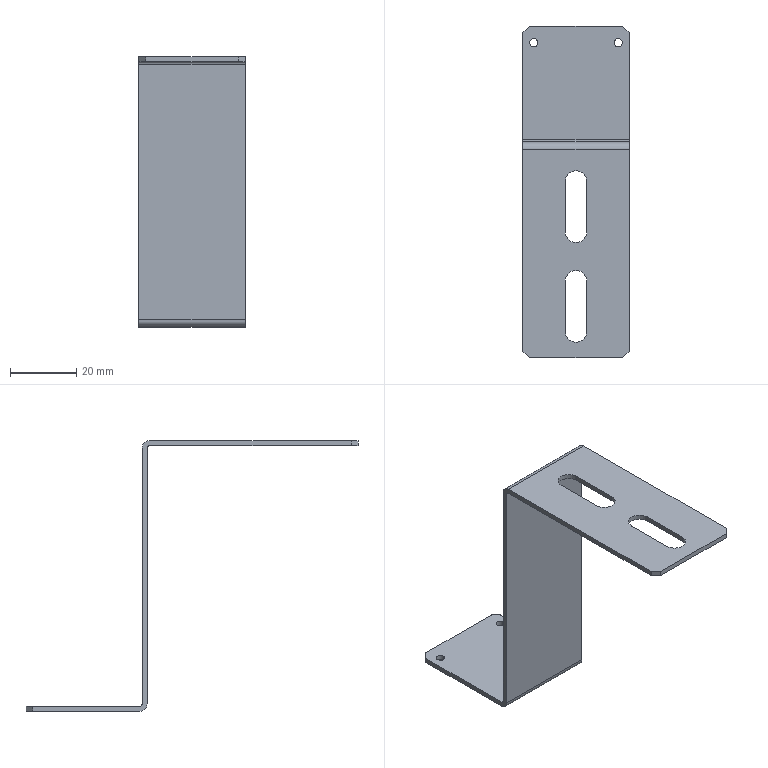Part | SolidWorks | features BaseBody 1 | 1 solid | 30 faces | box 32 x 100 x 81.5 mm | volume 8152 mm3 | plane 18 | cylinder 12 | commonest cylinder face diameters 2.5 x4 6.6 x4 1.473 x2 4.473 x2
STEP:
#1=CARTESIAN_POINT('',(11.45,95.,-80.));
#2=VERTEX_POINT('',#1);
#3=CARTESIAN_POINT('',(13.95,95.,-80.));
#4=VERTEX_POINT('',#3);
#5=CARTESIAN_POINT('',(12.7,95.,-80.));
#6=DIRECTION('',(0.,0.,1.));
#7=DIRECTION('',(1.,0.,0.));
#8=AXIS2_PLACEMENT_3D('',#5,#6,#7);
#9=CIRCLE('',#8,1.25);
#10=EDGE_CURVE('',#2,#4,#9,.T.);
#11=ORIENTED_EDGE('',*,*,#10,.T.);
#12=CARTESIAN_POINT('',(13.95,95.,-81.5));
#13=VERTEX_POINT('',#12);
#14=CARTESIAN_POINT('',(13.95,95.,-81.5));
#15=DIRECTION('',(0.,0.,-1.));
#16=VECTOR('',#15,1000.);
#17=LINE('',#14,#16);
#18=EDGE_CURVE('',#4,#13,#17,.T.);
#19=ORIENTED_EDGE('',*,*,#18,.T.);
#20=CARTESIAN_POINT('',(11.45,95.,-81.5));
#21=VERTEX_POINT('',#20);
#22=CARTESIAN_POINT('',(12.7,95.,-81.5));
#23=DIRECTION('',(0.,0.,-1.));
#24=DIRECTION('',(-1.,0.,0.));
#25=AXIS2_PLACEMENT_3D('',#22,#23,#24);
#26=CIRCLE('',#25,1.25);
#27=EDGE_CURVE('',#13,#21,#26,.T.);
#28=ORIENTED_EDGE('',*,*,#27,.T.);
#29=CARTESIAN_POINT('',(11.45,95.,-81.5));
#30=DIRECTION('',(0.,0.,-1.));
#31=VECTOR('',#30,1000.);
#32=LINE('',#29,#31);
#33=EDGE_CURVE('',#2,#21,#32,.T.);
#34=ORIENTED_EDGE('',*,*,#33,.F.);
#35=EDGE_LOOP('',(#11,#19,#28,#34));
#36=FACE_OUTER_BOUND('',#35,.T.);
#37=CARTESIAN_POINT('',(12.7,95.,-81.5));
#38=DIRECTION('',(0.,0.,-1.));
#39=DIRECTION('',(-1.,0.,0.));
#40=AXIS2_PLACEMENT_3D('',#37,#38,#39);
#41=CYLINDRICAL_SURFACE('',#40,1.25);
#42=ADVANCED_FACE('',(#36),#41,.F.);
#43=CARTESIAN_POINT('',(-13.95,95.,-80.));
#44=VERTEX_POINT('',#43);
#45=CARTESIAN_POINT('',(-11.45,95.,-80.));
#46=VERTEX_POINT('',#45);
#47=CARTESIAN_POINT('',(-12.7,95.,-80.));
#48=DIRECTION('',(0.,0.,1.));
#49=DIRECTION('',(1.,0.,0.));
#50=AXIS2_PLACEMENT_3D('',#47,#48,#49);
#51=CIRCLE('',#50,1.25);
#52=EDGE_CURVE('',#44,#46,#51,.T.);
#53=ORIENTED_EDGE('',*,*,#52,.T.);
#54=CARTESIAN_POINT('',(-11.45,95.,-81.5));
#55=VERTEX_POINT('',#54);
#56=CARTESIAN_POINT('',(-11.45,95.,-81.5));
#57=DIRECTION('',(0.,0.,-1.));
#58=VECTOR('',#57,1000.);
#59=LINE('',#56,#58);
#60=EDGE_CURVE('',#46,#55,#59,.T.);
#61=ORIENTED_EDGE('',*,*,#60,.T.);
#62=CARTESIAN_POINT('',(-13.95,95.,-81.5));
#63=VERTEX_POINT('',#62);
#64=CARTESIAN_POINT('',(-12.7,95.,-81.5));
#65=DIRECTION('',(0.,0.,-1.));
#66=DIRECTION('',(-1.,0.,0.));
#67=AXIS2_PLACEMENT_3D('',#64,#65,#66);
#68=CIRCLE('',#67,1.25);
#69=EDGE_CURVE('',#55,#63,#68,.T.);
#70=ORIENTED_EDGE('',*,*,#69,.T.);
#71=CARTESIAN_POINT('',(-13.95,95.,-81.5));
#72=DIRECTION('',(0.,0.,-1.));
#73=VECTOR('',#72,1000.);
#74=LINE('',#71,#73);
#75=EDGE_CURVE('',#44,#63,#74,.T.);
#76=ORIENTED_EDGE('',*,*,#75,.F.);
#77=EDGE_LOOP('',(#53,#61,#70,#76));
#78=FACE_OUTER_BOUND('',#77,.T.);
#79=CARTESIAN_POINT('',(-12.7,95.,-81.5));
#80=DIRECTION('',(0.,0.,-1.));
#81=DIRECTION('',(-1.,0.,0.));
#82=AXIS2_PLACEMENT_3D('',#79,#80,#81);
#83=CYLINDRICAL_SURFACE('',#82,1.25);
#84=ADVANCED_FACE('',(#78),#83,.F.);
#85=CARTESIAN_POINT('',(16.,98.,-80.));
#86=VERTEX_POINT('',#85);
#87=CARTESIAN_POINT('',(14.,100.,-80.));
#88=VERTEX_POINT('',#87);
#89=CARTESIAN_POINT('',(32.5,81.5,-80.));
#90=DIRECTION('',(-0.7071,0.7071,0.));
#91=VECTOR('',#90,1000.);
#92=LINE('',#89,#91);
#93=EDGE_CURVE('',#86,#88,#92,.T.);
#94=ORIENTED_EDGE('',*,*,#93,.F.);
#95=CARTESIAN_POINT('',(16.,98.,-81.5));
#96=VERTEX_POINT('',#95);
#97=CARTESIAN_POINT('',(16.,98.,-79.263));
#98=DIRECTION('',(0.,0.,1.));
#99=VECTOR('',#98,1000.);
#100=LINE('',#97,#99);
#101=EDGE_CURVE('',#96,#86,#100,.T.);
#102=ORIENTED_EDGE('',*,*,#101,.F.);
#103=CARTESIAN_POINT('',(14.,100.,-81.5));
#104=VERTEX_POINT('',#103);
#105=CARTESIAN_POINT('',(14.,100.,-81.5));
#106=DIRECTION('',(0.7071,-0.7071,0.));
#107=VECTOR('',#106,1000.);
#108=LINE('',#105,#107);
#109=EDGE_CURVE('',#104,#96,#108,.T.);
#110=ORIENTED_EDGE('',*,*,#109,.F.);
#111=CARTESIAN_POINT('',(14.,100.,-80.));
#112=DIRECTION('',(0.,0.,-1.));
#113=VECTOR('',#112,1000.);
#114=LINE('',#111,#113);
#115=EDGE_CURVE('',#88,#104,#114,.T.);
#116=ORIENTED_EDGE('',*,*,#115,.F.);
#117=EDGE_LOOP('',(#94,#102,#110,#116));
#118=FACE_OUTER_BOUND('',#117,.T.);
#119=CARTESIAN_POINT('',(14.,100.,-80.));
#120=DIRECTION('',(-0.7071,-0.7071,0.));
#121=DIRECTION('',(-0.7071,0.7071,0.));
#122=AXIS2_PLACEMENT_3D('',#119,#120,#121);
#123=PLANE('',#122);
#124=ADVANCED_FACE('',(#118),#123,.F.);
#125=CARTESIAN_POINT('',(-14.,100.,-80.));
#126=VERTEX_POINT('',#125);
#127=CARTESIAN_POINT('',(-16.,98.,-80.));
#128=VERTEX_POINT('',#127);
#129=CARTESIAN_POINT('',(-16.5,97.5,-80.));
#130=DIRECTION('',(-0.7071,-0.7071,0.));
#131=VECTOR('',#130,1000.);
#132=LINE('',#129,#131);
#133=EDGE_CURVE('',#126,#128,#132,.T.);
#134=ORIENTED_EDGE('',*,*,#133,.F.);
#135=CARTESIAN_POINT('',(-14.,100.,-81.5));
#136=VERTEX_POINT('',#135);
#137=CARTESIAN_POINT('',(-14.,100.,-80.));
#138=DIRECTION('',(0.,0.,1.));
#139=VECTOR('',#138,1000.);
#140=LINE('',#137,#139);
#141=EDGE_CURVE('',#136,#126,#140,.T.);
#142=ORIENTED_EDGE('',*,*,#141,.F.);
#143=CARTESIAN_POINT('',(-16.,98.,-81.5));
#144=VERTEX_POINT('',#143);
#145=CARTESIAN_POINT('',(-16.,98.,-81.5));
#146=DIRECTION('',(0.7071,0.7071,0.));
#147=VECTOR('',#146,1000.);
#148=LINE('',#145,#147);
#149=EDGE_CURVE('',#144,#136,#148,.T.);
#150=ORIENTED_EDGE('',*,*,#149,.F.);
#151=CARTESIAN_POINT('',(-16.,98.,-79.263));
#152=DIRECTION('',(0.,0.,-1.));
#153=VECTOR('',#152,1000.);
#154=LINE('',#151,#153);
#155=EDGE_CURVE('',#128,#144,#154,.T.);
#156=ORIENTED_EDGE('',*,*,#155,.F.);
#157=EDGE_LOOP('',(#134,#142,#150,#156));
#158=FACE_OUTER_BOUND('',#157,.T.);
#159=CARTESIAN_POINT('',(-16.,98.,-79.263));
#160=DIRECTION('',(0.7071,-0.7071,0.));
#161=DIRECTION('',(0.,0.,-1.));
#162=AXIS2_PLACEMENT_3D('',#159,#160,#161);
#163=PLANE('',#162);
#164=ADVANCED_FACE('',(#158),#163,.F.);
#165=CARTESIAN_POINT('',(-14.,0.,-1.5));
#166=VERTEX_POINT('',#165);
#167=CARTESIAN_POINT('',(-16.,2.,-1.5));
#168=VERTEX_POINT('',#167);
#169=CARTESIAN_POINT('',(-16.,2.,-1.5));
#170=DIRECTION('',(-0.7071,0.7071,0.));
#171=VECTOR('',#170,1000.);
#172=LINE('',#169,#171);
#173=EDGE_CURVE('',#166,#168,#172,.T.);
#174=ORIENTED_EDGE('',*,*,#173,.F.);
#175=CARTESIAN_POINT('',(-14.,0.,0.));
#176=VERTEX_POINT('',#175);
#177=CARTESIAN_POINT('',(-14.,0.,-1.5));
#178=DIRECTION('',(0.,0.,-1.));
#179=VECTOR('',#178,1000.);
#180=LINE('',#177,#179);
#181=EDGE_CURVE('',#176,#166,#180,.T.);
#182=ORIENTED_EDGE('',*,*,#181,.F.);
#183=CARTESIAN_POINT('',(-16.,2.,0.));
#184=VERTEX_POINT('',#183);
#185=CARTESIAN_POINT('',(1.,-15.,0.));
#186=DIRECTION('',(0.7071,-0.7071,0.));
#187=VECTOR('',#186,1000.);
#188=LINE('',#185,#187);
#189=EDGE_CURVE('',#184,#176,#188,.T.);
#190=ORIENTED_EDGE('',*,*,#189,.F.);
#191=CARTESIAN_POINT('',(-16.,2.,-2.237));
#192=DIRECTION('',(0.,0.,1.));
#193=VECTOR('',#192,1000.);
#194=LINE('',#191,#193);
#195=EDGE_CURVE('',#168,#184,#194,.T.);
#196=ORIENTED_EDGE('',*,*,#195,.F.);
#197=EDGE_LOOP('',(#174,#182,#190,#196));
#198=FACE_OUTER_BOUND('',#197,.T.);
#199=CARTESIAN_POINT('',(-16.,2.,-2.237));
#200=DIRECTION('',(0.7071,0.7071,0.));
#201=DIRECTION('',(0.,0.,-1.));
#202=AXIS2_PLACEMENT_3D('',#199,#200,#201);
#203=PLANE('',#202);
#204=ADVANCED_FACE('',(#198),#203,.F.);
#205=CARTESIAN_POINT('',(16.,2.,-1.5));
#206=VERTEX_POINT('',#205);
#207=CARTESIAN_POINT('',(14.,0.,-1.5));
#208=VERTEX_POINT('',#207);
#209=CARTESIAN_POINT('',(14.,0.,-1.5));
#210=DIRECTION('',(-0.7071,-0.7071,0.));
#211=VECTOR('',#210,1000.);
#212=LINE('',#209,#211);
#213=EDGE_CURVE('',#206,#208,#212,.T.);
#214=ORIENTED_EDGE('',*,*,#213,.F.);
#215=CARTESIAN_POINT('',(16.,2.,0.));
#216=VERTEX_POINT('',#215);
#217=CARTESIAN_POINT('',(16.,2.,-1.5));
#218=DIRECTION('',(0.,0.,-1.));
#219=VECTOR('',#218,1000.);
#220=LINE('',#217,#219);
#221=EDGE_CURVE('',#216,#206,#220,.T.);
#222=ORIENTED_EDGE('',*,*,#221,.F.);
#223=CARTESIAN_POINT('',(14.,0.,0.));
#224=VERTEX_POINT('',#223);
#225=CARTESIAN_POINT('',(15.,1.,0.));
#226=DIRECTION('',(0.7071,0.7071,0.));
#227=VECTOR('',#226,1000.);
#228=LINE('',#225,#227);
#229=EDGE_CURVE('',#224,#216,#228,.T.);
#230=ORIENTED_EDGE('',*,*,#229,.F.);
#231=CARTESIAN_POINT('',(14.,0.,0.));
#232=DIRECTION('',(0.,0.,1.));
#233=VECTOR('',#232,1000.);
#234=LINE('',#231,#233);
#235=EDGE_CURVE('',#208,#224,#234,.T.);
#236=ORIENTED_EDGE('',*,*,#235,.F.);
#237=EDGE_LOOP('',(#214,#222,#230,#236));
#238=FACE_OUTER_BOUND('',#237,.T.);
#239=CARTESIAN_POINT('',(14.,0.,-1.5));
#240=DIRECTION('',(0.7071,-0.7071,0.));
#241=DIRECTION('',(0.,0.,-1.));
#242=AXIS2_PLACEMENT_3D('',#239,#240,#241);
#243=PLANE('',#242);
#244=ADVANCED_FACE('',(#238),#243,.T.);
#245=CARTESIAN_POINT('',(-3.3,38.,0.));
#246=VERTEX_POINT('',#245);
#247=CARTESIAN_POINT('',(-3.3,38.,-1.5));
#248=VERTEX_POINT('',#247);
#249=CARTESIAN_POINT('',(-3.3,38.,0.001));
#250=DIRECTION('',(0.,0.,-1.));
#251=VECTOR('',#250,1000.);
#252=LINE('',#249,#251);
#253=EDGE_CURVE('',#246,#248,#252,.T.);
#254=ORIENTED_EDGE('',*,*,#253,.T.);
#255=CARTESIAN_POINT('',(-3.3,53.,-1.5));
#256=VERTEX_POINT('',#255);
#257=CARTESIAN_POINT('',(-3.3,38.,-1.5));
#258=DIRECTION('',(0.,1.,0.));
#259=VECTOR('',#258,1000.);
#260=LINE('',#257,#259);
#261=EDGE_CURVE('',#248,#256,#260,.T.);
#262=ORIENTED_EDGE('',*,*,#261,.T.);
#263=CARTESIAN_POINT('',(-3.3,53.,0.));
#264=VERTEX_POINT('',#263);
#265=CARTESIAN_POINT('',(-3.3,53.,0.001));
#266=DIRECTION('',(0.,0.,-1.));
#267=VECTOR('',#266,1000.);
#268=LINE('',#265,#267);
#269=EDGE_CURVE('',#264,#256,#268,.T.);
#270=ORIENTED_EDGE('',*,*,#269,.F.);
#271=CARTESIAN_POINT('',(-3.3,38.,0.));
#272=DIRECTION('',(0.,1.,0.));
#273=VECTOR('',#272,1000.);
#274=LINE('',#271,#273);
#275=EDGE_CURVE('',#246,#264,#274,.T.);
#276=ORIENTED_EDGE('',*,*,#275,.F.);
#277=EDGE_LOOP('',(#254,#262,#270,#276));
#278=FACE_OUTER_BOUND('',#277,.T.);
#279=CARTESIAN_POINT('',(-3.3,38.,0.001));
#280=DIRECTION('',(-1.,0.,0.));
#281=DIRECTION('',(0.,0.,1.));
#282=AXIS2_PLACEMENT_3D('',#279,#280,#281);
#283=PLANE('',#282);
#284=ADVANCED_FACE('',(#278),#283,.F.);
#285=ORIENTED_EDGE('',*,*,#269,.T.);
#286=CARTESIAN_POINT('',(3.3,53.,-1.5));
#287=VERTEX_POINT('',#286);
#288=CARTESIAN_POINT('',(0.,53.,-1.5));
#289=DIRECTION('',(0.,0.,-1.));
#290=DIRECTION('',(-1.,0.,0.));
#291=AXIS2_PLACEMENT_3D('',#288,#289,#290);
#292=CIRCLE('',#291,3.3);
#293=EDGE_CURVE('',#256,#287,#292,.T.);
#294=ORIENTED_EDGE('',*,*,#293,.T.);
#295=CARTESIAN_POINT('',(3.3,53.,0.));
#296=VERTEX_POINT('',#295);
#297=CARTESIAN_POINT('',(3.3,53.,0.001));
#298=DIRECTION('',(0.,0.,-1.));
#299=VECTOR('',#298,1000.);
#300=LINE('',#297,#299);
#301=EDGE_CURVE('',#296,#287,#300,.T.);
#302=ORIENTED_EDGE('',*,*,#301,.F.);
#303=CARTESIAN_POINT('',(0.,53.,0.));
#304=DIRECTION('',(0.,0.,-1.));
#305=DIRECTION('',(1.,0.,0.));
#306=AXIS2_PLACEMENT_3D('',#303,#304,#305);
#307=CIRCLE('',#306,3.3);
#308=EDGE_CURVE('',#264,#296,#307,.T.);
#309=ORIENTED_EDGE('',*,*,#308,.F.);
#310=EDGE_LOOP('',(#285,#294,#302,#309));
#311=FACE_OUTER_BOUND('',#310,.T.);
#312=CARTESIAN_POINT('',(0.,53.,0.001));
#313=DIRECTION('',(0.,0.,-1.));
#314=DIRECTION('',(-1.,0.,0.));
#315=AXIS2_PLACEMENT_3D('',#312,#313,#314);
#316=CYLINDRICAL_SURFACE('',#315,3.3);
#317=ADVANCED_FACE('',(#311),#316,.F.);
#318=ORIENTED_EDGE('',*,*,#301,.T.);
#319=CARTESIAN_POINT('',(3.3,38.,-1.5));
#320=VERTEX_POINT('',#319);
#321=CARTESIAN_POINT('',(3.3,38.,-1.5));
#322=DIRECTION('',(0.,-1.,0.));
#323=VECTOR('',#322,1000.);
#324=LINE('',#321,#323);
#325=EDGE_CURVE('',#287,#320,#324,.T.);
#326=ORIENTED_EDGE('',*,*,#325,.T.);
#327=CARTESIAN_POINT('',(3.3,38.,0.));
#328=VERTEX_POINT('',#327);
#329=CARTESIAN_POINT('',(3.3,38.,0.001));
#330=DIRECTION('',(0.,0.,-1.));
#331=VECTOR('',#330,1000.);
#332=LINE('',#329,#331);
#333=EDGE_CURVE('',#328,#320,#332,.T.);
#334=ORIENTED_EDGE('',*,*,#333,.F.);
#335=CARTESIAN_POINT('',(3.3,38.,0.));
#336=DIRECTION('',(0.,-1.,0.));
#337=VECTOR('',#336,1000.);
#338=LINE('',#335,#337);
#339=EDGE_CURVE('',#296,#328,#338,.T.);
#340=ORIENTED_EDGE('',*,*,#339,.F.);
#341=EDGE_LOOP('',(#318,#326,#334,#340));
#342=FACE_OUTER_BOUND('',#341,.T.);
#343=CARTESIAN_POINT('',(3.3,38.,0.001));
#344=DIRECTION('',(1.,0.,0.));
#345=DIRECTION('',(0.,1.,0.));
#346=AXIS2_PLACEMENT_3D('',#343,#344,#345);
#347=PLANE('',#346);
#348=ADVANCED_FACE('',(#342),#347,.F.);
#349=ORIENTED_EDGE('',*,*,#333,.T.);
#350=CARTESIAN_POINT('',(0.,38.,-1.5));
#351=DIRECTION('',(0.,0.,-1.));
#352=DIRECTION('',(-1.,0.,0.));
#353=AXIS2_PLACEMENT_3D('',#350,#351,#352);
#354=CIRCLE('',#353,3.3);
#355=EDGE_CURVE('',#320,#248,#354,.T.);
#356=ORIENTED_EDGE('',*,*,#355,.T.);
#357=ORIENTED_EDGE('',*,*,#253,.F.);
#358=CARTESIAN_POINT('',(0.,38.,0.));
#359=DIRECTION('',(0.,0.,-1.));
#360=DIRECTION('',(1.,0.,0.));
#361=AXIS2_PLACEMENT_3D('',#358,#359,#360);
#362=CIRCLE('',#361,3.3);
#363=EDGE_CURVE('',#328,#246,#362,.T.);
#364=ORIENTED_EDGE('',*,*,#363,.F.);
#365=EDGE_LOOP('',(#349,#356,#357,#364));
#366=FACE_OUTER_BOUND('',#365,.T.);
#367=CARTESIAN_POINT('',(0.,38.,0.001));
#368=DIRECTION('',(0.,0.,-1.));
#369=DIRECTION('',(-1.,0.,0.));
#370=AXIS2_PLACEMENT_3D('',#367,#368,#369);
#371=CYLINDRICAL_SURFACE('',#370,3.3);
#372=ADVANCED_FACE('',(#366),#371,.F.);
#373=CARTESIAN_POINT('',(-3.3,8.,0.));
#374=VERTEX_POINT('',#373);
#375=CARTESIAN_POINT('',(-3.3,8.,-1.5));
#376=VERTEX_POINT('',#375);
#377=CARTESIAN_POINT('',(-3.3,8.,0.001));
#378=DIRECTION('',(0.,0.,-1.));
#379=VECTOR('',#378,1000.);
#380=LINE('',#377,#379);
#381=EDGE_CURVE('',#374,#376,#380,.T.);
#382=ORIENTED_EDGE('',*,*,#381,.T.);
#383=CARTESIAN_POINT('',(-3.3,23.,-1.5));
#384=VERTEX_POINT('',#383);
#385=CARTESIAN_POINT('',(-3.3,8.,-1.5));
#386=DIRECTION('',(0.,1.,0.));
#387=VECTOR('',#386,1000.);
#388=LINE('',#385,#387);
#389=EDGE_CURVE('',#376,#384,#388,.T.);
#390=ORIENTED_EDGE('',*,*,#389,.T.);
#391=CARTESIAN_POINT('',(-3.3,23.,0.));
#392=VERTEX_POINT('',#391);
#393=CARTESIAN_POINT('',(-3.3,23.,0.001));
#394=DIRECTION('',(0.,0.,-1.));
#395=VECTOR('',#394,1000.);
#396=LINE('',#393,#395);
#397=EDGE_CURVE('',#392,#384,#396,.T.);
#398=ORIENTED_EDGE('',*,*,#397,.F.);
#399=CARTESIAN_POINT('',(-3.3,8.,0.));
#400=DIRECTION('',(0.,1.,0.));
#401=VECTOR('',#400,1000.);
#402=LINE('',#399,#401);
#403=EDGE_CURVE('',#374,#392,#402,.T.);
#404=ORIENTED_EDGE('',*,*,#403,.F.);
#405=EDGE_LOOP('',(#382,#390,#398,#404));
#406=FACE_OUTER_BOUND('',#405,.T.);
#407=CARTESIAN_POINT('',(-3.3,8.,0.001));
#408=DIRECTION('',(-1.,0.,0.));
#409=DIRECTION('',(0.,0.,1.));
#410=AXIS2_PLACEMENT_3D('',#407,#408,#409);
#411=PLANE('',#410);
#412=ADVANCED_FACE('',(#406),#411,.F.);
#413=ORIENTED_EDGE('',*,*,#397,.T.);
#414=CARTESIAN_POINT('',(3.3,23.,-1.5));
#415=VERTEX_POINT('',#414);
#416=CARTESIAN_POINT('',(0.,23.,-1.5));
#417=DIRECTION('',(0.,0.,-1.));
#418=DIRECTION('',(-1.,0.,0.));
#419=AXIS2_PLACEMENT_3D('',#416,#417,#418);
#420=CIRCLE('',#419,3.3);
#421=EDGE_CURVE('',#384,#415,#420,.T.);
#422=ORIENTED_EDGE('',*,*,#421,.T.);
#423=CARTESIAN_POINT('',(3.3,23.,0.));
#424=VERTEX_POINT('',#423);
#425=CARTESIAN_POINT('',(3.3,23.,0.001));
#426=DIRECTION('',(0.,0.,-1.));
#427=VECTOR('',#426,1000.);
#428=LINE('',#425,#427);
#429=EDGE_CURVE('',#424,#415,#428,.T.);
#430=ORIENTED_EDGE('',*,*,#429,.F.);
#431=CARTESIAN_POINT('',(0.,23.,0.));
#432=DIRECTION('',(0.,0.,-1.));
#433=DIRECTION('',(1.,0.,0.));
#434=AXIS2_PLACEMENT_3D('',#431,#432,#433);
#435=CIRCLE('',#434,3.3);
#436=EDGE_CURVE('',#392,#424,#435,.T.);
#437=ORIENTED_EDGE('',*,*,#436,.F.);
#438=EDGE_LOOP('',(#413,#422,#430,#437));
#439=FACE_OUTER_BOUND('',#438,.T.);
#440=CARTESIAN_POINT('',(0.,23.,0.001));
#441=DIRECTION('',(0.,0.,-1.));
#442=DIRECTION('',(-1.,0.,0.));
#443=AXIS2_PLACEMENT_3D('',#440,#441,#442);
#444=CYLINDRICAL_SURFACE('',#443,3.3);
#445=ADVANCED_FACE('',(#439),#444,.F.);
#446=ORIENTED_EDGE('',*,*,#429,.T.);
#447=CARTESIAN_POINT('',(3.3,8.,-1.5));
#448=VERTEX_POINT('',#447);
#449=CARTESIAN_POINT('',(3.3,8.,-1.5));
#450=DIRECTION('',(0.,-1.,0.));
#451=VECTOR('',#450,1000.);
#452=LINE('',#449,#451);
#453=EDGE_CURVE('',#415,#448,#452,.T.);
#454=ORIENTED_EDGE('',*,*,#453,.T.);
#455=CARTESIAN_POINT('',(3.3,8.,0.));
#456=VERTEX_POINT('',#455);
#457=CARTESIAN_POINT('',(3.3,8.,0.001));
#458=DIRECTION('',(0.,0.,-1.));
#459=VECTOR('',#458,1000.);
#460=LINE('',#457,#459);
#461=EDGE_CURVE('',#456,#448,#460,.T.);
#462=ORIENTED_EDGE('',*,*,#461,.F.);
#463=CARTESIAN_POINT('',(3.3,8.,0.));
#464=DIRECTION('',(0.,-1.,0.));
#465=VECTOR('',#464,1000.);
#466=LINE('',#463,#465);
#467=EDGE_CURVE('',#424,#456,#466,.T.);
#468=ORIENTED_EDGE('',*,*,#467,.F.);
#469=EDGE_LOOP('',(#446,#454,#462,#468));
#470=FACE_OUTER_BOUND('',#469,.T.);
#471=CARTESIAN_POINT('',(3.3,8.,0.001));
#472=DIRECTION('',(1.,0.,0.));
#473=DIRECTION('',(0.,1.,0.));
#474=AXIS2_PLACEMENT_3D('',#471,#472,#473);
#475=PLANE('',#474);
#476=ADVANCED_FACE('',(#470),#475,.F.);
#477=ORIENTED_EDGE('',*,*,#461,.T.);
#478=CARTESIAN_POINT('',(0.,8.,-1.5));
#479=DIRECTION('',(0.,0.,-1.));
#480=DIRECTION('',(-1.,0.,0.));
#481=AXIS2_PLACEMENT_3D('',#478,#479,#480);
#482=CIRCLE('',#481,3.3);
#483=EDGE_CURVE('',#448,#376,#482,.T.);
#484=ORIENTED_EDGE('',*,*,#483,.T.);
#485=ORIENTED_EDGE('',*,*,#381,.F.);
#486=CARTESIAN_POINT('',(0.,8.,0.));
#487=DIRECTION('',(0.,0.,-1.));
#488=DIRECTION('',(1.,0.,0.));
#489=AXIS2_PLACEMENT_3D('',#486,#487,#488);
#490=CIRCLE('',#489,3.3);
#491=EDGE_CURVE('',#456,#374,#490,.T.);
#492=ORIENTED_EDGE('',*,*,#491,.F.);
#493=EDGE_LOOP('',(#477,#484,#485,#492));
#494=FACE_OUTER_BOUND('',#493,.T.);
#495=CARTESIAN_POINT('',(0.,8.,0.001));
#496=DIRECTION('',(0.,0.,-1.));
#497=DIRECTION('',(-1.,0.,0.));
#498=AXIS2_PLACEMENT_3D('',#495,#496,#497);
#499=CYLINDRICAL_SURFACE('',#498,3.3);
#500=ADVANCED_FACE('',(#494),#499,.F.);
#501=CARTESIAN_POINT('',(-16.,63.5,-79.263));
#502=VERTEX_POINT('',#501);
#503=CARTESIAN_POINT('',(-16.,65.737,-81.5));
#504=VERTEX_POINT('',#503);
#505=CARTESIAN_POINT('',(-16.,65.737,-79.263));
#506=DIRECTION('',(1.,0.,0.));
#507=DIRECTION('',(0.,0.,-1.));
#508=AXIS2_PLACEMENT_3D('',#505,#506,#507);
#509=CIRCLE('',#508,2.237);
#510=EDGE_CURVE('',#502,#504,#509,.T.);
#511=ORIENTED_EDGE('',*,*,#510,.T.);
#512=CARTESIAN_POINT('',(16.,65.737,-81.5));
#513=VERTEX_POINT('',#512);
#514=CARTESIAN_POINT('',(16.,65.737,-81.5));
#515=DIRECTION('',(-1.,0.,0.));
#516=VECTOR('',#515,1000.);
#517=LINE('',#514,#516);
#518=EDGE_CURVE('',#513,#504,#517,.T.);
#519=ORIENTED_EDGE('',*,*,#518,.F.);
#520=CARTESIAN_POINT('',(16.,63.5,-79.263));
#521=VERTEX_POINT('',#520);
#522=CARTESIAN_POINT('',(16.,65.737,-79.263));
#523=DIRECTION('',(1.,0.,0.));
#524=DIRECTION('',(0.,0.,-1.));
#525=AXIS2_PLACEMENT_3D('',#522,#523,#524);
#526=CIRCLE('',#525,2.237);
#527=EDGE_CURVE('',#521,#513,#526,.T.);
#528=ORIENTED_EDGE('',*,*,#527,.F.);
#529=CARTESIAN_POINT('',(16.,63.5,-79.263));
#530=DIRECTION('',(-1.,0.,0.));
#531=VECTOR('',#530,1000.);
#532=LINE('',#529,#531);
#533=EDGE_CURVE('',#521,#502,#532,.T.);
#534=ORIENTED_EDGE('',*,*,#533,.T.);
#535=EDGE_LOOP('',(#511,#519,#528,#534));
#536=FACE_OUTER_BOUND('',#535,.T.);
#537=CARTESIAN_POINT('',(16.,65.737,-79.263));
#538=DIRECTION('',(-1.,0.,0.));
#539=DIRECTION('',(0.,0.,1.));
#540=AXIS2_PLACEMENT_3D('',#537,#538,#539);
#541=CYLINDRICAL_SURFACE('',#540,2.237);
#542=ADVANCED_FACE('',(#536),#541,.T.);
#543=CARTESIAN_POINT('',(-16.,63.5,-2.237));
#544=VERTEX_POINT('',#543);
#545=CARTESIAN_POINT('',(-16.,63.5,0.));
#546=DIRECTION('',(0.,0.,-1.));
#547=VECTOR('',#546,1000.);
#548=LINE('',#545,#547);
#549=EDGE_CURVE('',#544,#502,#548,.T.);
#550=ORIENTED_EDGE('',*,*,#549,.T.);
#551=ORIENTED_EDGE('',*,*,#533,.F.);
#552=CARTESIAN_POINT('',(16.,63.5,-2.237));
#553=VERTEX_POINT('',#552);
#554=CARTESIAN_POINT('',(16.,63.5,0.));
#555=DIRECTION('',(0.,0.,-1.));
#556=VECTOR('',#555,1000.);
#557=LINE('',#554,#556);
#558=EDGE_CURVE('',#553,#521,#557,.T.);
#559=ORIENTED_EDGE('',*,*,#558,.F.);
#560=CARTESIAN_POINT('',(16.,63.5,-2.237));
#561=DIRECTION('',(-1.,0.,0.));
#562=VECTOR('',#561,1000.);
#563=LINE('',#560,#562);
#564=EDGE_CURVE('',#553,#544,#563,.T.);
#565=ORIENTED_EDGE('',*,*,#564,.T.);
#566=EDGE_LOOP('',(#550,#551,#559,#565));
#567=FACE_OUTER_BOUND('',#566,.T.);
#568=CARTESIAN_POINT('',(16.,63.5,0.));
#569=DIRECTION('',(0.,1.,0.));
#570=DIRECTION('',(1.,0.,0.));
#571=AXIS2_PLACEMENT_3D('',#568,#569,#570);
#572=PLANE('',#571);
#573=ADVANCED_FACE('',(#567),#572,.F.);
#574=CARTESIAN_POINT('',(-16.,62.763,-1.5));
#575=VERTEX_POINT('',#574);
#576=CARTESIAN_POINT('',(-16.,62.763,-2.237));
#577=DIRECTION('',(-1.,0.,0.));
#578=DIRECTION('',(0.,0.,-1.));
#579=AXIS2_PLACEMENT_3D('',#576,#577,#578);
#580=CIRCLE('',#579,0.7366);
#581=EDGE_CURVE('',#575,#544,#580,.T.);
#582=ORIENTED_EDGE('',*,*,#581,.T.);
#583=ORIENTED_EDGE('',*,*,#564,.F.);
#584=CARTESIAN_POINT('',(16.,62.763,-1.5));
#585=VERTEX_POINT('',#584);
#586=CARTESIAN_POINT('',(16.,62.763,-2.237));
#587=DIRECTION('',(-1.,0.,0.));
#588=DIRECTION('',(0.,0.,-1.));
#589=AXIS2_PLACEMENT_3D('',#586,#587,#588);
#590=CIRCLE('',#589,0.7366);
#591=EDGE_CURVE('',#585,#553,#590,.T.);
#592=ORIENTED_EDGE('',*,*,#591,.F.);
#593=CARTESIAN_POINT('',(16.,62.763,-1.5));
#594=DIRECTION('',(-1.,0.,0.));
#595=VECTOR('',#594,1000.);
#596=LINE('',#593,#595);
#597=EDGE_CURVE('',#585,#575,#596,.T.);
#598=ORIENTED_EDGE('',*,*,#597,.T.);
#599=EDGE_LOOP('',(#582,#583,#592,#598));
#600=FACE_OUTER_BOUND('',#599,.T.);
#601=CARTESIAN_POINT('',(16.,62.763,-2.237));
#602=DIRECTION('',(-1.,0.,0.));
#603=DIRECTION('',(0.,0.,1.));
#604=AXIS2_PLACEMENT_3D('',#601,#602,#603);
#605=CYLINDRICAL_SURFACE('',#604,0.7366);
#606=ADVANCED_FACE('',(#600),#605,.F.);
#607=ORIENTED_EDGE('',*,*,#389,.F.);
#608=ORIENTED_EDGE('',*,*,#483,.F.);
#609=ORIENTED_EDGE('',*,*,#453,.F.);
#610=ORIENTED_EDGE('',*,*,#421,.F.);
#611=EDGE_LOOP('',(#607,#608,#609,#610));
#612=FACE_BOUND('',#611,.T.);
#613=ORIENTED_EDGE('',*,*,#261,.F.);
#614=ORIENTED_EDGE('',*,*,#355,.F.);
#615=ORIENTED_EDGE('',*,*,#325,.F.);
#616=ORIENTED_EDGE('',*,*,#293,.F.);
#617=EDGE_LOOP('',(#613,#614,#615,#616));
#618=FACE_BOUND('',#617,.T.);
#619=CARTESIAN_POINT('',(16.,0.,-1.5));
#620=DIRECTION('',(0.,1.,0.));
#621=VECTOR('',#620,1000.);
#622=LINE('',#619,#621);
#623=EDGE_CURVE('',#206,#585,#622,.T.);
#624=ORIENTED_EDGE('',*,*,#623,.F.);
#625=ORIENTED_EDGE('',*,*,#213,.T.);
#626=CARTESIAN_POINT('',(16.,0.,-1.5));
#627=DIRECTION('',(-1.,0.,0.));
#628=VECTOR('',#627,1000.);
#629=LINE('',#626,#628);
#630=EDGE_CURVE('',#208,#166,#629,.T.);
#631=ORIENTED_EDGE('',*,*,#630,.T.);
#632=ORIENTED_EDGE('',*,*,#173,.T.);
#633=CARTESIAN_POINT('',(-16.,0.,-1.5));
#634=DIRECTION('',(0.,1.,0.));
#635=VECTOR('',#634,1000.);
#636=LINE('',#633,#635);
#637=EDGE_CURVE('',#168,#575,#636,.T.);
#638=ORIENTED_EDGE('',*,*,#637,.T.);
#639=ORIENTED_EDGE('',*,*,#597,.F.);
#640=EDGE_LOOP('',(#624,#625,#631,#632,#638,#639));
#641=FACE_OUTER_BOUND('',#640,.T.);
#642=CARTESIAN_POINT('',(16.,0.,-1.5));
#643=DIRECTION('',(0.,0.,1.));
#644=DIRECTION('',(1.,0.,0.));
#645=AXIS2_PLACEMENT_3D('',#642,#643,#644);
#646=PLANE('',#645);
#647=ADVANCED_FACE('',(#612,#618,#641),#646,.F.);
#648=ORIENTED_EDGE('',*,*,#630,.F.);
#649=ORIENTED_EDGE('',*,*,#235,.T.);
#650=CARTESIAN_POINT('',(16.,0.,0.));
#651=DIRECTION('',(-1.,0.,0.));
#652=VECTOR('',#651,1000.);
#653=LINE('',#650,#652);
#654=EDGE_CURVE('',#224,#176,#653,.T.);
#655=ORIENTED_EDGE('',*,*,#654,.T.);
#656=ORIENTED_EDGE('',*,*,#181,.T.);
#657=EDGE_LOOP('',(#648,#649,#655,#656));
#658=FACE_OUTER_BOUND('',#657,.T.);
#659=CARTESIAN_POINT('',(16.,0.,-1.5));
#660=DIRECTION('',(0.,-1.,0.));
#661=DIRECTION('',(0.,0.,-1.));
#662=AXIS2_PLACEMENT_3D('',#659,#660,#661);
#663=PLANE('',#662);
#664=ADVANCED_FACE('',(#658),#663,.T.);
#665=ORIENTED_EDGE('',*,*,#491,.T.);
#666=ORIENTED_EDGE('',*,*,#403,.T.);
#667=ORIENTED_EDGE('',*,*,#436,.T.);
#668=ORIENTED_EDGE('',*,*,#467,.T.);
#669=EDGE_LOOP('',(#665,#666,#667,#668));
#670=FACE_BOUND('',#669,.T.);
#671=ORIENTED_EDGE('',*,*,#363,.T.);
#672=ORIENTED_EDGE('',*,*,#275,.T.);
#673=ORIENTED_EDGE('',*,*,#308,.T.);
#674=ORIENTED_EDGE('',*,*,#339,.T.);
#675=EDGE_LOOP('',(#671,#672,#673,#674));
#676=FACE_BOUND('',#675,.T.);
#677=ORIENTED_EDGE('',*,*,#654,.F.);
#678=ORIENTED_EDGE('',*,*,#229,.T.);
#679=CARTESIAN_POINT('',(16.,62.763,0.));
#680=VERTEX_POINT('',#679);
#681=CARTESIAN_POINT('',(16.,0.,0.));
#682=DIRECTION('',(0.,1.,0.));
#683=VECTOR('',#682,1000.);
#684=LINE('',#681,#683);
#685=EDGE_CURVE('',#216,#680,#684,.T.);
#686=ORIENTED_EDGE('',*,*,#685,.T.);
#687=CARTESIAN_POINT('',(-16.,62.763,0.));
#688=VERTEX_POINT('',#687);
#689=CARTESIAN_POINT('',(16.,62.763,0.));
#690=DIRECTION('',(-1.,0.,0.));
#691=VECTOR('',#690,1000.);
#692=LINE('',#689,#691);
#693=EDGE_CURVE('',#680,#688,#692,.T.);
#694=ORIENTED_EDGE('',*,*,#693,.T.);
#695=CARTESIAN_POINT('',(-16.,0.,0.));
#696=DIRECTION('',(0.,1.,0.));
#697=VECTOR('',#696,1000.);
#698=LINE('',#695,#697);
#699=EDGE_CURVE('',#184,#688,#698,.T.);
#700=ORIENTED_EDGE('',*,*,#699,.F.);
#701=ORIENTED_EDGE('',*,*,#189,.T.);
#702=EDGE_LOOP('',(#677,#678,#686,#694,#700,#701));
#703=FACE_OUTER_BOUND('',#702,.T.);
#704=CARTESIAN_POINT('',(16.,0.,0.));
#705=DIRECTION('',(0.,0.,1.));
#706=DIRECTION('',(1.,0.,0.));
#707=AXIS2_PLACEMENT_3D('',#704,#705,#706);
#708=PLANE('',#707);
#709=ADVANCED_FACE('',(#670,#676,#703),#708,.T.);
#710=CARTESIAN_POINT('',(-16.,65.,-2.237));
#711=VERTEX_POINT('',#710);
#712=CARTESIAN_POINT('',(-16.,62.763,-2.237));
#713=DIRECTION('',(-1.,0.,0.));
#714=DIRECTION('',(0.,0.,-1.));
#715=AXIS2_PLACEMENT_3D('',#712,#713,#714);
#716=CIRCLE('',#715,2.237);
#717=EDGE_CURVE('',#688,#711,#716,.T.);
#718=ORIENTED_EDGE('',*,*,#717,.F.);
#719=ORIENTED_EDGE('',*,*,#693,.F.);
#720=CARTESIAN_POINT('',(16.,65.,-2.237));
#721=VERTEX_POINT('',#720);
#722=CARTESIAN_POINT('',(16.,62.763,-2.237));
#723=DIRECTION('',(-1.,0.,0.));
#724=DIRECTION('',(0.,0.,-1.));
#725=AXIS2_PLACEMENT_3D('',#722,#723,#724);
#726=CIRCLE('',#725,2.237);
#727=EDGE_CURVE('',#680,#721,#726,.T.);
#728=ORIENTED_EDGE('',*,*,#727,.T.);
#729=CARTESIAN_POINT('',(16.,65.,-2.237));
#730=DIRECTION('',(-1.,0.,0.));
#731=VECTOR('',#730,1000.);
#732=LINE('',#729,#731);
#733=EDGE_CURVE('',#721,#711,#732,.T.);
#734=ORIENTED_EDGE('',*,*,#733,.T.);
#735=EDGE_LOOP('',(#718,#719,#728,#734));
#736=FACE_OUTER_BOUND('',#735,.T.);
#737=CARTESIAN_POINT('',(16.,62.763,-2.237));
#738=DIRECTION('',(-1.,0.,0.));
#739=DIRECTION('',(0.,0.,1.));
#740=AXIS2_PLACEMENT_3D('',#737,#738,#739);
#741=CYLINDRICAL_SURFACE('',#740,2.237);
#742=ADVANCED_FACE('',(#736),#741,.T.);
#743=CARTESIAN_POINT('',(-16.,65.,-79.263));
#744=VERTEX_POINT('',#743);
#745=CARTESIAN_POINT('',(-16.,65.,0.));
#746=DIRECTION('',(0.,0.,-1.));
#747=VECTOR('',#746,1000.);
#748=LINE('',#745,#747);
#749=EDGE_CURVE('',#711,#744,#748,.T.);
#750=ORIENTED_EDGE('',*,*,#749,.F.);
#751=ORIENTED_EDGE('',*,*,#733,.F.);
#752=CARTESIAN_POINT('',(16.,65.,-79.263));
#753=VERTEX_POINT('',#752);
#754=CARTESIAN_POINT('',(16.,65.,0.));
#755=DIRECTION('',(0.,0.,-1.));
#756=VECTOR('',#755,1000.);
#757=LINE('',#754,#756);
#758=EDGE_CURVE('',#721,#753,#757,.T.);
#759=ORIENTED_EDGE('',*,*,#758,.T.);
#760=CARTESIAN_POINT('',(16.,65.,-79.263));
#761=DIRECTION('',(-1.,0.,0.));
#762=VECTOR('',#761,1000.);
#763=LINE('',#760,#762);
#764=EDGE_CURVE('',#753,#744,#763,.T.);
#765=ORIENTED_EDGE('',*,*,#764,.T.);
#766=EDGE_LOOP('',(#750,#751,#759,#765));
#767=FACE_OUTER_BOUND('',#766,.T.);
#768=CARTESIAN_POINT('',(16.,65.,0.));
#769=DIRECTION('',(0.,1.,0.));
#770=DIRECTION('',(1.,0.,0.));
#771=AXIS2_PLACEMENT_3D('',#768,#769,#770);
#772=PLANE('',#771);
#773=ADVANCED_FACE('',(#767),#772,.T.);
#774=CARTESIAN_POINT('',(-16.,65.737,-80.));
#775=VERTEX_POINT('',#774);
#776=CARTESIAN_POINT('',(-16.,65.737,-79.263));
#777=DIRECTION('',(1.,0.,0.));
#778=DIRECTION('',(0.,0.,1.));
#779=AXIS2_PLACEMENT_3D('',#776,#777,#778);
#780=CIRCLE('',#779,0.7366);
#781=EDGE_CURVE('',#744,#775,#780,.T.);
#782=ORIENTED_EDGE('',*,*,#781,.F.);
#783=ORIENTED_EDGE('',*,*,#764,.F.);
#784=CARTESIAN_POINT('',(16.,65.737,-80.));
#785=VERTEX_POINT('',#784);
#786=CARTESIAN_POINT('',(16.,65.737,-79.263));
#787=DIRECTION('',(1.,0.,0.));
#788=DIRECTION('',(0.,0.,1.));
#789=AXIS2_PLACEMENT_3D('',#786,#787,#788);
#790=CIRCLE('',#789,0.7366);
#791=EDGE_CURVE('',#753,#785,#790,.T.);
#792=ORIENTED_EDGE('',*,*,#791,.T.);
#793=CARTESIAN_POINT('',(16.,65.737,-80.));
#794=DIRECTION('',(-1.,0.,0.));
#795=VECTOR('',#794,1000.);
#796=LINE('',#793,#795);
#797=EDGE_CURVE('',#785,#775,#796,.T.);
#798=ORIENTED_EDGE('',*,*,#797,.T.);
#799=EDGE_LOOP('',(#782,#783,#792,#798));
#800=FACE_OUTER_BOUND('',#799,.T.);
#801=CARTESIAN_POINT('',(16.,65.737,-79.263));
#802=DIRECTION('',(-1.,0.,0.));
#803=DIRECTION('',(0.,0.,1.));
#804=AXIS2_PLACEMENT_3D('',#801,#802,#803);
#805=CYLINDRICAL_SURFACE('',#804,0.7366);
#806=ADVANCED_FACE('',(#800),#805,.F.);
#807=ORIENTED_EDGE('',*,*,#52,.F.);
#808=CARTESIAN_POINT('',(-12.7,95.,-80.));
#809=DIRECTION('',(0.,0.,1.));
#810=DIRECTION('',(1.,0.,0.));
#811=AXIS2_PLACEMENT_3D('',#808,#809,#810);
#812=CIRCLE('',#811,1.25);
#813=EDGE_CURVE('',#46,#44,#812,.T.);
#814=ORIENTED_EDGE('',*,*,#813,.F.);
#815=EDGE_LOOP('',(#807,#814));
#816=FACE_BOUND('',#815,.T.);
#817=ORIENTED_EDGE('',*,*,#10,.F.);
#818=CARTESIAN_POINT('',(12.7,95.,-80.));
#819=DIRECTION('',(0.,0.,1.));
#820=DIRECTION('',(1.,0.,0.));
#821=AXIS2_PLACEMENT_3D('',#818,#819,#820);
#822=CIRCLE('',#821,1.25);
#823=EDGE_CURVE('',#4,#2,#822,.T.);
#824=ORIENTED_EDGE('',*,*,#823,.F.);
#825=EDGE_LOOP('',(#817,#824));
#826=FACE_BOUND('',#825,.T.);
#827=CARTESIAN_POINT('',(16.,100.,-80.));
#828=DIRECTION('',(-1.,0.,0.));
#829=VECTOR('',#828,1000.);
#830=LINE('',#827,#829);
#831=EDGE_CURVE('',#88,#126,#830,.T.);
#832=ORIENTED_EDGE('',*,*,#831,.T.);
#833=ORIENTED_EDGE('',*,*,#133,.T.);
#834=CARTESIAN_POINT('',(-16.,65.,-80.));
#835=DIRECTION('',(0.,1.,0.));
#836=VECTOR('',#835,1000.);
#837=LINE('',#834,#836);
#838=EDGE_CURVE('',#775,#128,#837,.T.);
#839=ORIENTED_EDGE('',*,*,#838,.F.);
#840=ORIENTED_EDGE('',*,*,#797,.F.);
#841=CARTESIAN_POINT('',(16.,65.,-80.));
#842=DIRECTION('',(0.,1.,0.));
#843=VECTOR('',#842,1000.);
#844=LINE('',#841,#843);
#845=EDGE_CURVE('',#785,#86,#844,.T.);
#846=ORIENTED_EDGE('',*,*,#845,.T.);
#847=ORIENTED_EDGE('',*,*,#93,.T.);
#848=EDGE_LOOP('',(#832,#833,#839,#840,#846,#847));
#849=FACE_OUTER_BOUND('',#848,.T.);
#850=CARTESIAN_POINT('',(16.,65.,-80.));
#851=DIRECTION('',(0.,0.,1.));
#852=DIRECTION('',(1.,0.,0.));
#853=AXIS2_PLACEMENT_3D('',#850,#851,#852);
#854=PLANE('',#853);
#855=ADVANCED_FACE('',(#816,#826,#849),#854,.T.);
#856=CARTESIAN_POINT('',(16.,100.,-81.5));
#857=DIRECTION('',(-1.,0.,0.));
#858=VECTOR('',#857,1000.);
#859=LINE('',#856,#858);
#860=EDGE_CURVE('',#104,#136,#859,.T.);
#861=ORIENTED_EDGE('',*,*,#860,.T.);
#862=ORIENTED_EDGE('',*,*,#141,.T.);
#863=ORIENTED_EDGE('',*,*,#831,.F.);
#864=ORIENTED_EDGE('',*,*,#115,.T.);
#865=EDGE_LOOP('',(#861,#862,#863,#864));
#866=FACE_OUTER_BOUND('',#865,.T.);
#867=CARTESIAN_POINT('',(16.,100.,-80.));
#868=DIRECTION('',(0.,1.,0.));
#869=DIRECTION('',(1.,0.,0.));
#870=AXIS2_PLACEMENT_3D('',#867,#868,#869);
#871=PLANE('',#870);
#872=ADVANCED_FACE('',(#866),#871,.T.);
#873=CARTESIAN_POINT('',(-12.7,95.,-81.5));
#874=DIRECTION('',(0.,0.,-1.));
#875=DIRECTION('',(-1.,0.,0.));
#876=AXIS2_PLACEMENT_3D('',#873,#874,#875);
#877=CIRCLE('',#876,1.25);
#878=EDGE_CURVE('',#63,#55,#877,.T.);
#879=ORIENTED_EDGE('',*,*,#878,.F.);
#880=ORIENTED_EDGE('',*,*,#69,.F.);
#881=EDGE_LOOP('',(#879,#880));
#882=FACE_BOUND('',#881,.T.);
#883=CARTESIAN_POINT('',(12.7,95.,-81.5));
#884=DIRECTION('',(0.,0.,-1.));
#885=DIRECTION('',(-1.,0.,0.));
#886=AXIS2_PLACEMENT_3D('',#883,#884,#885);
#887=CIRCLE('',#886,1.25);
#888=EDGE_CURVE('',#21,#13,#887,.T.);
#889=ORIENTED_EDGE('',*,*,#888,.F.);
#890=ORIENTED_EDGE('',*,*,#27,.F.);
#891=EDGE_LOOP('',(#889,#890));
#892=FACE_BOUND('',#891,.T.);
#893=CARTESIAN_POINT('',(-16.,65.,-81.5));
#894=DIRECTION('',(0.,1.,0.));
#895=VECTOR('',#894,1000.);
#896=LINE('',#893,#895);
#897=EDGE_CURVE('',#504,#144,#896,.T.);
#898=ORIENTED_EDGE('',*,*,#897,.T.);
#899=ORIENTED_EDGE('',*,*,#149,.T.);
#900=ORIENTED_EDGE('',*,*,#860,.F.);
#901=ORIENTED_EDGE('',*,*,#109,.T.);
#902=CARTESIAN_POINT('',(16.,65.,-81.5));
#903=DIRECTION('',(0.,1.,0.));
#904=VECTOR('',#903,1000.);
#905=LINE('',#902,#904);
#906=EDGE_CURVE('',#513,#96,#905,.T.);
#907=ORIENTED_EDGE('',*,*,#906,.F.);
#908=ORIENTED_EDGE('',*,*,#518,.T.);
#909=EDGE_LOOP('',(#898,#899,#900,#901,#907,#908));
#910=FACE_OUTER_BOUND('',#909,.T.);
#911=CARTESIAN_POINT('',(16.,65.,-81.5));
#912=DIRECTION('',(0.,0.,1.));
#913=DIRECTION('',(1.,0.,0.));
#914=AXIS2_PLACEMENT_3D('',#911,#912,#913);
#915=PLANE('',#914);
#916=ADVANCED_FACE('',(#882,#892,#910),#915,.F.);
#917=ORIENTED_EDGE('',*,*,#581,.F.);
#918=ORIENTED_EDGE('',*,*,#637,.F.);
#919=ORIENTED_EDGE('',*,*,#195,.T.);
#920=ORIENTED_EDGE('',*,*,#699,.T.);
#921=ORIENTED_EDGE('',*,*,#717,.T.);
#922=ORIENTED_EDGE('',*,*,#749,.T.);
#923=ORIENTED_EDGE('',*,*,#781,.T.);
#924=ORIENTED_EDGE('',*,*,#838,.T.);
#925=ORIENTED_EDGE('',*,*,#155,.T.);
#926=ORIENTED_EDGE('',*,*,#897,.F.);
#927=ORIENTED_EDGE('',*,*,#510,.F.);
#928=ORIENTED_EDGE('',*,*,#549,.F.);
#929=EDGE_LOOP('',(#917,#918,#919,#920,#921,#922,#923,#924,#925,#926,#927,#928));
#930=FACE_OUTER_BOUND('',#929,.T.);
#931=CARTESIAN_POINT('',(-16.,62.763,0.));
#932=DIRECTION('',(-1.,0.,0.));
#933=DIRECTION('',(0.,0.,1.));
#934=AXIS2_PLACEMENT_3D('',#931,#932,#933);
#935=PLANE('',#934);
#936=ADVANCED_FACE('',(#930),#935,.T.);
#937=ORIENTED_EDGE('',*,*,#591,.T.);
#938=ORIENTED_EDGE('',*,*,#558,.T.);
#939=ORIENTED_EDGE('',*,*,#527,.T.);
#940=ORIENTED_EDGE('',*,*,#906,.T.);
#941=ORIENTED_EDGE('',*,*,#101,.T.);
#942=ORIENTED_EDGE('',*,*,#845,.F.);
#943=ORIENTED_EDGE('',*,*,#791,.F.);
#944=ORIENTED_EDGE('',*,*,#758,.F.);
#945=ORIENTED_EDGE('',*,*,#727,.F.);
#946=ORIENTED_EDGE('',*,*,#685,.F.);
#947=ORIENTED_EDGE('',*,*,#221,.T.);
#948=ORIENTED_EDGE('',*,*,#623,.T.);
#949=EDGE_LOOP('',(#937,#938,#939,#940,#941,#942,#943,#944,#945,#946,#947,#948));
#950=FACE_OUTER_BOUND('',#949,.T.);
#951=CARTESIAN_POINT('',(16.,65.,-2.237));
#952=DIRECTION('',(1.,0.,0.));
#953=DIRECTION('',(0.,1.,0.));
#954=AXIS2_PLACEMENT_3D('',#951,#952,#953);
#955=PLANE('',#954);
#956=ADVANCED_FACE('',(#950),#955,.T.);
#957=ORIENTED_EDGE('',*,*,#60,.F.);
#958=ORIENTED_EDGE('',*,*,#813,.T.);
#959=ORIENTED_EDGE('',*,*,#75,.T.);
#960=ORIENTED_EDGE('',*,*,#878,.T.);
#961=EDGE_LOOP('',(#957,#958,#959,#960));
#962=FACE_OUTER_BOUND('',#961,.T.);
#963=CARTESIAN_POINT('',(-12.7,95.,-81.5));
#964=DIRECTION('',(0.,0.,-1.));
#965=DIRECTION('',(-1.,0.,0.));
#966=AXIS2_PLACEMENT_3D('',#963,#964,#965);
#967=CYLINDRICAL_SURFACE('',#966,1.25);
#968=ADVANCED_FACE('',(#962),#967,.F.);
#969=ORIENTED_EDGE('',*,*,#18,.F.);
#970=ORIENTED_EDGE('',*,*,#823,.T.);
#971=ORIENTED_EDGE('',*,*,#33,.T.);
#972=ORIENTED_EDGE('',*,*,#888,.T.);
#973=EDGE_LOOP('',(#969,#970,#971,#972));
#974=FACE_OUTER_BOUND('',#973,.T.);
#975=CARTESIAN_POINT('',(12.7,95.,-81.5));
#976=DIRECTION('',(0.,0.,-1.));
#977=DIRECTION('',(-1.,0.,0.));
#978=AXIS2_PLACEMENT_3D('',#975,#976,#977);
#979=CYLINDRICAL_SURFACE('',#978,1.25);
#980=ADVANCED_FACE('',(#974),#979,.F.);
#981=CLOSED_SHELL('',(#42,#84,#124,#164,#204,#244,#284,#317,#348,#372,#412,#445,#476,#500,#542,#573,#606,#647,#664,#709,#742,#773,#806,#855,#872,#916,#936,#956,#968,#980));
#982=MANIFOLD_SOLID_BREP('',#981);
#983=CARTESIAN_POINT('',(0.,0.,0.));
#984=DIRECTION('',(0.,0.,1.));
#985=DIRECTION('',(1.,0.,0.));
#986=AXIS2_PLACEMENT_3D('',#983,#984,#985);
#987=(LENGTH_UNIT()NAMED_UNIT(*)SI_UNIT(.MILLI.,.METRE.));
#988=UNCERTAINTY_MEASURE_WITH_UNIT(LENGTH_MEASURE(0.00001),#987,'','');
#989=(NAMED_UNIT(*)PLANE_ANGLE_UNIT()SI_UNIT($,.RADIAN.));
#990=(NAMED_UNIT(*)SI_UNIT($,.STERADIAN.)SOLID_ANGLE_UNIT());
#991=(GEOMETRIC_REPRESENTATION_CONTEXT(3)GLOBAL_UNCERTAINTY_ASSIGNED_CONTEXT((#988))GLOBAL_UNIT_ASSIGNED_CONTEXT((#987,#989,#990))REPRESENTATION_CONTEXT('',''));
#992=ADVANCED_BREP_SHAPE_REPRESENTATION('',(#982,#986),#991);